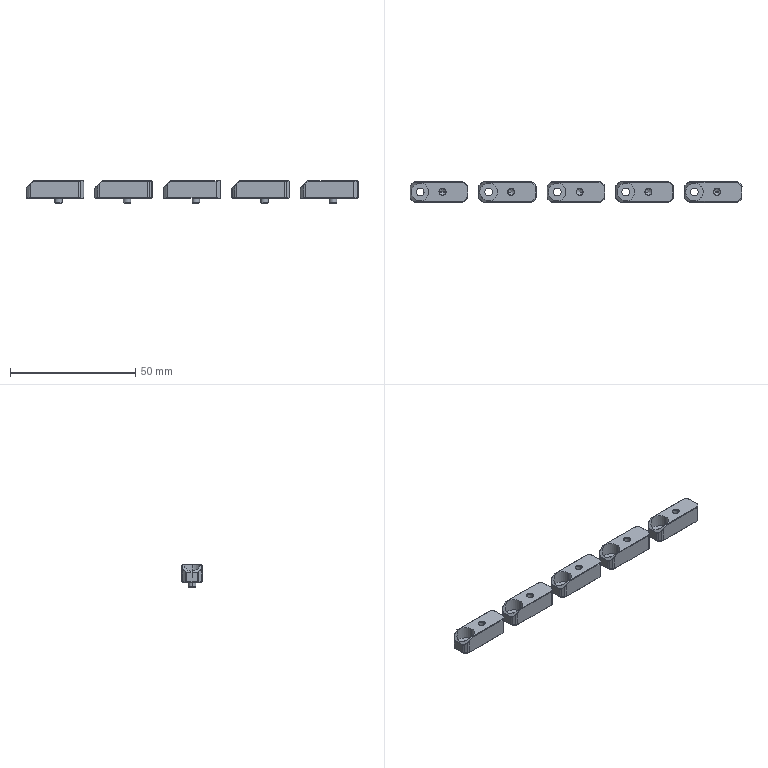NC program | NX | posted by the shop | part box 132.6 x 8 x 8.9 mm
Whole program:
%
G40 G17 G49 G80 G90
M05
M09
G91 G28 Z0.0
M01
T01 M06
S5500 M03
(ToolName=D10J-25L-35L D.=10.00 R.=0.00)
 (0.15)(1.00)
G00 G90 G54 X-15.568 Y-9.358
T02
G43 Z20. H01 M08
Z1.15
G01 X-15.418 Y-9.348 Z.213 F2500.
X-15.269 Y-9.338 Z-.158
X-15.119 Y-9.328 Z-.43
X-14.969 Y-9.318 Z-.65
X-14.82 Y-9.308 Z-.834
X-14.67 Y-9.298 Z-.992
X-14.52 Y-9.288 Z-1.13
X-14.371 Y-9.278 Z-1.25
X-14.221 Y-9.268 Z-1.355
X-14.071 Y-9.258 Z-1.448
X-13.922 Y-9.248 Z-1.529
X-13.772 Y-9.238 Z-1.6
X-13.622 Y-9.228 Z-1.66
X-13.473 Y-9.218 Z-1.712
X-13.323 Y-9.208 Z-1.755
X-13.173 Y-9.198 Z-1.789
X-13.024 Y-9.187 Z-1.816
X-12.874 Y-9.177 Z-1.835
X-12.724 Y-9.167 Z-1.846
X-12.575 Y-9.157 Z-1.85
X-10.906 Y-9.045
G03 X-10.068 Y-8.486 I-.068 J1.009
X-9.547 Y-6.515 I-5.399 J2.482
X-9.233 Y-.391 I-54.139 J5.843
G01 X-9.192 Y11.158
G02 X-7.172 Y14.937 I5.526 J-.525
X-2.877 Y16.974 I6.278 J-7.689
X2.78 Y17.563 I5.379 J-24.206
X6.58 Y15.381 I-.7 J-5.619
X8.523 Y11.04 I-8.162 J-6.259
X9.114 Y5.178 I-32.253 J-6.21
X9.187 Y-11.22 I-609.076 J-10.924
X7.123 Y-14.978 I-5.557 J.607
X2.718 Y-17.01 I-6.311 J7.89
X-2.743 Y-17.566 I-5.329 J25.259
X-6.557 Y-15.409 I.651 J5.601
X-8.546 Y-10.061 I7.386 J5.791
X-8.576 Y-5.963 I41.357 J2.349
G03 X-8.391 Y8.56 I-496.759 J13.586
G02 X-5.338 Y14.057 I7.315 J-.466
X-.198 Y16.126 I6.51 J-8.752
X4.995 Y13.989 I.367 J-6.486
X7.419 Y9.435 I-7.893 J-7.123
X8.242 Y3.503 I-27.14 J-6.788
X8.379 Y-8.694 I-236.972 J-8.767
X5.299 Y-14.081 I-7.33 J.617
X.224 Y-16.122 I-6.487 J8.801
X-5.265 Y-13.58 I-.398 J6.338
X-7.205 Y-8.918 I8.504 J6.274
X-7.618 Y-3.239 I33.864 J5.318
X-7.577 Y6.665 I356.761 J3.47
X-3.211 Y13.522 I8.185 J-.394
X2.776 Y12.95 I2.499 J-5.461
X5.992 Y8.808 I-5.31 J-7.442
X7.254 Y3.271 I-18.248 J-7.07
X7.553 Y-6.72 I-93.712 J-7.807
X3.235 Y-13.5 I-8.158 J.43
X-2.544 Y-12.897 I-2.382 J5.168
X-5.576 Y-8.744 I5.221 J6.996
X-6.606 Y-3.462 I18.15 J6.281
X-6.753 Y5.033 I86.712 J5.747
X-5.478 Y9.195 I8.615 J-.364
X-.113 Y11.199 I4.112 J-2.826
X3.987 Y8.335 I-1.784 J-6.921
X6.034 Y3.372 I-10.567 J-7.262
X6.541 Y-.392 I-31.249 J-6.119
G01 X6.589 Y-.601
G02 X6.684 Y-5.109 I-46.458 J-3.237
X5.5 Y-9.093 I-8.338 J.31
X.672 Y-10.972 I-3.804 J2.634
X-3.378 Y-8.239 I1.486 J6.57
X-4.397 Y-6.52 I10.563 J7.422
G01 X-5.336 Y-5.469
X-5.978 Y-4.412
X-6.414 Y-3.255
X-6.628 Y-2.038
X-6.613 Y-.801
G03 X-6.103 Y3.097 I-24.535 J5.19
G02 X-5.681 Y5.349 I8.073 J-.349
X-2.146 Y7.745 I3.689 J-1.638
X2.217 Y6.08 I.237 J-5.929
X3.941 Y3.873 I-6.653 J-6.975
G03 X4.313 Y3.562 I1.669 J1.613
G01 X5.159 Y2.696
X5.835 Y1.69
X6.316 Y.579
X6.589 Y-.601
X6.643 Y-1.811
G02 X5.983 Y-4.953 I-16.172 J1.756
X3.647 Y-7.046 I-3.405 J1.45
X-.001 Y-8.15 I-3.719 J5.709
G01 X-1.233 Y-8.035
X-2.422 Y-7.693
X-3.526 Y-7.138
G02 X-4.576 Y-6.313 I8.815 J12.301
G03 X-6.078 Y-7.634 I-.743 J-.669
G01 X-5.891 Y-7.852
X-4.606 Y-9.347 Z-1.75
X-3.739 Y-10.356 F10000.
G03 X-3.428 Y-10.599 I.802 J.707
G01 X-2.744 Y-10.943
X-2.054 Y-11.273
G03 X-.003 Y-11.525 I1.489 J3.649
G01 X1.275 Y-11.344
X2.552 Y-11.147
G03 X6.785 Y-8.838 I-1.546 J7.868
G01 X8.694 Y-6.853
G03 X8.955 Y-5.969 I-.722 J.694
G01 X8.642 Y-4.349
X8.388 Y-3.065 Z-1.816 F2500.
X8.334 Y-2.846 Z-1.828
X8.208 Y-2.658 Z-1.839
X8.025 Y-2.526 Z-1.85
G03 X6.476 Y-3.011 I-.6 J-.8
G01 X6.095 Y-4.16
X5.511 Y-5.222
X4.745 Y-6.159
X3.821 Y-6.943
G02 X-.001 Y-8.15 I-3.908 J5.719
G01 X-1.233 Y-8.035
X-2.422 Y-7.693
X-3.526 Y-7.138
X-4.509 Y-6.388
X-5.336 Y-5.469
X-5.978 Y-4.412
X-6.414 Y-3.255
X-6.628 Y-2.038
X-6.613 Y-.801
X-6.369 Y.411
G02 X-5.7 Y1.971 I11.124 J-3.85
X-4.43 Y3.459 I8.873 J-6.284
G01 X-3.451 Y4.184
X-2.357 Y4.718
X-1.183 Y5.044
X.03 Y5.15
G02 X2.282 Y4.746 I-.226 J-7.739
G01 X3.323 Y4.26
X4.14 Y3.684
G03 X5.549 Y5.055 I.577 J.817
G01 X5.194 Y5.477 Z-1.822
X4.828 Y5.887 Z-1.794
X4.252 Y6.541 Z-1.75
X2.992 Y7.969 F10000.
X2.718 Y8.246
X2.433 Y8.512
G03 X1.51 Y8.759 I-.759 J-.992
G01 X.352 Y8.607
X-.803 Y8.44
G03 X-4.877 Y6.917 I2.057 J-11.716
G01 X-7.181 Y5.531
G03 X-7.661 Y4.77 I.517 J-.858
G01 X-7.816 Y3.161
X-7.958 Y1.651 Z-1.827 F2500.
X-7.969 Y1.419 Z-1.838
X-7.872 Y1.209 Z-1.85
G03 X-6.033 Y1.246 I.912 J.411
G01 X-5.914 Y1.541
X-5.27 Y2.553
G03 X-5.273 Y3.642 I-.853 J.542
G01 X-6.236 Y5.137
X-6.317 Y5.263 Z-1.846
X-6.399 Y5.389 Z-1.835
X-6.48 Y5.515 Z-1.816
X-6.561 Y5.641 Z-1.789
X-6.642 Y5.767 Z-1.755
X-6.724 Y5.893 Z-1.712
X-6.805 Y6.019 Z-1.66
X-6.886 Y6.145 Z-1.6
X-6.967 Y6.271 Z-1.529
X-7.049 Y6.397 Z-1.448
X-7.13 Y6.524 Z-1.355
X-7.211 Y6.65 Z-1.25
X-7.292 Y6.776 Z-1.13
X-7.374 Y6.902 Z-.992
X-7.455 Y7.028 Z-.834
X-7.536 Y7.154 Z-.65
X-7.617 Y7.28 Z-.43
X-7.699 Y7.406 Z-.158
X-7.78 Y7.532 Z.213
X-7.861 Y7.658 Z1.15
G00 Z20.
X.8 Y-13.733
Z3.13
G01 X.794 Y-13.583 Z2.193
X.787 Y-13.433 Z1.822
X.78 Y-13.283 Z1.55
X.773 Y-13.133 Z1.33
X.766 Y-12.984 Z1.146
X.759 Y-12.834 Z.988
X.753 Y-12.684 Z.85
X.746 Y-12.534 Z.73
X.739 Y-12.384 Z.625
X.732 Y-12.234 Z.532
X.725 Y-12.084 Z.451
X.718 Y-11.935 Z.38
X.712 Y-11.785 Z.32
X.705 Y-11.635 Z.268
X.698 Y-11.485 Z.225
X.691 Y-11.335 Z.191
X.684 Y-11.185 Z.164
X.677 Y-11.036 Z.145
X.671 Y-10.886 Z.134
X.664 Y-10.736 Z.13
X.59 Y-9.106
G03 X-.008 Y-8.229 I-1.01 J-.046
G02 X-1.137 Y-7.72 I15.465 J35.789
G01 X-2.388 Y-7.357
X-3.476 Y-6.784
X-4.432 Y-6.012
X-5.221 Y-5.07
X-5.813 Y-3.993
X-6.185 Y-2.822
X-6.324 Y-1.6
X-6.224 Y-.376
G02 X-5.465 Y1.683 I7.206 J-1.486
X-4.049 Y3.359 I6.265 J-3.859
X-2.146 Y4.45 I4.57 J-5.767
X.016 Y4.825 I2.325 J-6.981
X3.823 Y3.539 I-.106 J-6.592
G01 X4.666 Y2.769
X5.358 Y1.861
X5.875 Y.843
X6.2 Y-.251
X6.324 Y-1.386
X6.241 Y-2.525
X5.955 Y-3.63
X5.475 Y-4.666
X4.817 Y-5.598
X4.002 Y-6.398
G02 X2.091 Y-7.469 I-4.575 J5.919
X.014 Y-7.825 I-2.267 J6.994
G01 X-1.21 Y-7.708
G03 X-2.17 Y-8.19 I-.096 J-1.006
G01 X-3.096 Y-9.717
X-3.174 Y-9.845 Z.134
X-3.252 Y-9.974 Z.145
X-3.329 Y-10.102 Z.164
X-3.407 Y-10.23 Z.191
X-3.485 Y-10.358 Z.225
X-3.563 Y-10.487 Z.268
X-3.64 Y-10.615 Z.32
X-3.718 Y-10.743 Z.38
X-3.796 Y-10.872 Z.451
X-3.874 Y-11. Z.532
X-3.951 Y-11.128 Z.625
X-4.029 Y-11.256 Z.73
X-4.107 Y-11.385 Z.85
X-4.185 Y-11.513 Z.988
X-4.262 Y-11.641 Z1.146
X-4.34 Y-11.769 Z1.33
X-4.418 Y-11.898 Z1.55
X-4.496 Y-12.026 Z1.822
X-4.573 Y-12.154 Z2.193
X-4.651 Y-12.283 Z3.13
G00 Z20.
X-2.407 Y-13.103
Z3.15
G01 X-2.384 Y-12.954 Z2.213
X-2.362 Y-12.806 Z1.842
X-2.34 Y-12.658 Z1.57
X-2.317 Y-12.509 Z1.35
X-2.295 Y-12.361 Z1.166
X-2.273 Y-12.213 Z1.008
X-2.25 Y-12.064 Z.87
X-2.228 Y-11.916 Z.75
X-2.206 Y-11.768 Z.645
X-2.184 Y-11.619 Z.552
X-2.161 Y-11.471 Z.471
X-2.139 Y-11.323 Z.4
X-2.117 Y-11.174 Z.34
X-2.094 Y-11.026 Z.288
X-2.072 Y-10.878 Z.245
X-2.05 Y-10.729 Z.211
X-2.027 Y-10.581 Z.184
X-2.005 Y-10.433 Z.165
X-1.983 Y-10.284 Z.154
X-1.96 Y-10.136 Z.15
X-1.694 Y-8.367
G03 X-1.96 Y-7.521 I-1.001 J.15
G02 X-4.029 Y-4.566 I5.409 J5.987
X-3.877 Y-.884 I4.118 J1.675
X-3.211 Y-.011 I6.028 J-3.91
G01 X-3.117 Y.106 Z.154
X-3.023 Y.223 Z.165
X-2.929 Y.34 Z.184
X-2.835 Y.457 Z.211
X-2.741 Y.574 Z.245
X-2.647 Y.691 Z.288
X-2.553 Y.808 Z.34
X-2.459 Y.924 Z.4
X-2.365 Y1.041 Z.471
X-2.271 Y1.158 Z.552
X-2.177 Y1.275 Z.645
X-2.083 Y1.392 Z.75
X-1.989 Y1.509 Z.87
X-1.895 Y1.626 Z1.008
X-1.801 Y1.743 Z1.166
X-1.707 Y1.86 Z1.35
X-1.613 Y1.977 Z1.57
X-1.519 Y2.094 Z1.842
X-1.425 Y2.21 Z2.213
X-1.331 Y2.327 Z3.15
G00 Z20.
M05
M09
G91 G28 Z0.0
M01
T02 M06
S4500 M03
(ToolName=4J-10L-25L D.=4.00 R.=0.00)
 (0.00)(0.00)
G00 G90 G54 X0.0 Y-6.75
T04
G43 Z20. H02 M08
Z3.
G01 Z0.0 F800.
Y-2.75
Y-.25
Y3.75
Z3.
G00 Z20.
G00 X8. Y5.55 S4500 M03
Z1.
G01 Z-2. F800.
X4.
Y-9.586
G02 X3.707 Y-10.293 I-1. J0.0
G01 X2.793 Y-11.207
G02 X2.086 Y-11.5 I-.707 J.707
G01 X-2.086
G02 X-2.793 Y-11.207 I0.0 J1.
G01 X-3.707 Y-10.293
G02 X-4. Y-9.586 I.707 J.707
G01 Y-5.095
X-1.6
G03 X1.6 I1.6 J3.595
G01 Y-9.006
X1.506 Y-9.1
X-1.506
X-1.6 Y-9.006
Y-5.095
X-4.
Y9.586
G02 X-3.707 Y10.293 I1. J0.0
G01 X-2.793 Y11.207
G02 X-2.086 Y11.5 I.707 J-.707
G01 X2.086
G02 X2.793 Y11.207 I0.0 J-1.
G01 X3.707 Y10.293
G02 X4. Y9.586 I-.707 J-.707
G01 Y5.55
X1.6
Y2.095
G03 X-1.6 I-1.6 J-3.595
G01 X-1.405 Y1.656
G02 I1.405 J-3.156
G01 X-1.6 Y2.095
Y9.006
X-1.506 Y9.1
X1.506
X1.6 Y9.006
Y5.55
X8.
Z1.
G00 Z20.
M05
M09
G91 G28 Z0.0
M01
T04 M06
S3500 M03
(ToolName=D8 spot drill D.=8.00 R.=0.00)
 (0.00)(0.00)
G00 G90 G54 X-1. Y2.25
T08
G43 Z20. H04 M08
Z1.5
G01 Z-1.5 F800.
G03 X0.0 Y1.25 I1. J0.0
G02 I0.0 J-2.75
G03 X1. Y2.25 I0.0 J1.
G01 Z1.5
G00 Z20.
G00 X-6.3 Y-10.586 S3500 M03
Z-.5
G01 Z-3.5 F800.
G03 X-5.3 Y-9.586 I0.0 J1.
G01 Y9.586
G02 X-4.626 Y11.212 I2.3 J0.0
G01 X-3.712 Y12.126
G02 X-2.086 Y12.8 I1.626 J-1.626
G01 X2.086
G02 X3.712 Y12.126 I0.0 J-2.3
G01 X4.626 Y11.212
G02 X5.3 Y9.586 I-1.626 J-1.626
G01 Y-9.586
G02 X4.626 Y-11.212 I-2.3 J0.0
G01 X3.712 Y-12.126
G02 X2.086 Y-12.8 I-1.626 J1.626
G01 X-2.086
G02 X-3.712 Y-12.126 I0.0 J2.3
G01 X-4.626 Y-11.212
G02 X-5.3 Y-9.586 I1.626 J1.626
G03 X-6.3 Y-8.586 I-1. J0.0
G01 Z-.5
G00 Z20.
G00 X0.0 Y7.5 S2500 M03
G98 G82 X0.0 Y7.5 Z-3.6 R1. F200.
G80
G00 Z20.
M05
M09
G91 G28 Z0.0
M01
T08 M06
S2500 M03
(ToolName=drill D3.2 D.=3.20 R.=0.00)
 (0.00)(0.00)
G00 G90 G54 X0.0 Y7.5
T01
G43 Z20. H08 M08
G98 G82 X0.0 Y7.5 Z-7. R1. F200.
G80
G00 Z20.
M05
M09
G91 G28 Z0.0
G28 Y0.0
M30
(The Sum of Machine Time:0.62 Minutes)
%